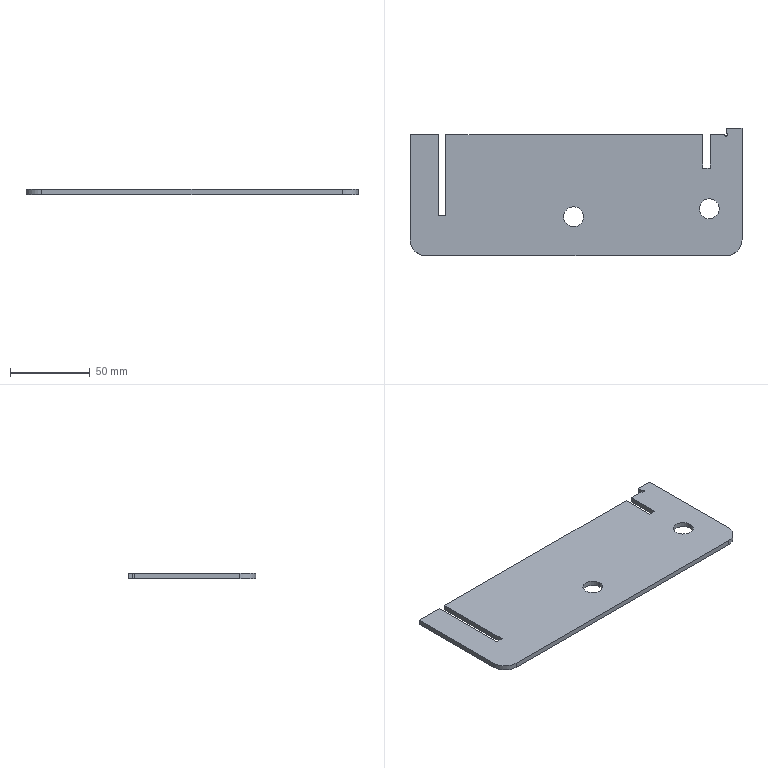Part | SolidWorks | features FlatPattern 1, SMBaseFlange 1, SheetMetal 1 | 1 solid | 23 faces | box 208 x 80 x 3.2 mm | volume 48747 mm3 | plane 16 | cylinder 7 | commonest cylinder face diameters 12.5 x4 20 x2 2 x1
STEP:
#1=CARTESIAN_POINT('',(88.351,-1041.506,3.2));
#2=VERTEX_POINT('',#1);
#3=CARTESIAN_POINT('',(100.851,-1041.506,3.2));
#4=VERTEX_POINT('',#3);
#5=CARTESIAN_POINT('',(94.601,-1041.506,3.2));
#6=DIRECTION('',(0.,0.,1.));
#7=DIRECTION('',(1.,0.,0.));
#8=AXIS2_PLACEMENT_3D('',#5,#6,#7);
#9=CIRCLE('',#8,6.25);
#10=EDGE_CURVE('',#2,#4,#9,.T.);
#11=ORIENTED_EDGE('',*,*,#10,.T.);
#12=CARTESIAN_POINT('',(100.851,-1041.506,0.));
#13=VERTEX_POINT('',#12);
#14=CARTESIAN_POINT('',(100.851,-1041.506,3.2));
#15=DIRECTION('',(0.,0.,-1.));
#16=VECTOR('',#15,1000.);
#17=LINE('',#14,#16);
#18=EDGE_CURVE('',#4,#13,#17,.T.);
#19=ORIENTED_EDGE('',*,*,#18,.T.);
#20=CARTESIAN_POINT('',(88.351,-1041.506,0.));
#21=VERTEX_POINT('',#20);
#22=CARTESIAN_POINT('',(94.601,-1041.506,0.));
#23=DIRECTION('',(0.,0.,1.));
#24=DIRECTION('',(1.,0.,0.));
#25=AXIS2_PLACEMENT_3D('',#22,#23,#24);
#26=CIRCLE('',#25,6.25);
#27=EDGE_CURVE('',#21,#13,#26,.T.);
#28=ORIENTED_EDGE('',*,*,#27,.F.);
#29=CARTESIAN_POINT('',(88.351,-1041.506,3.2));
#30=DIRECTION('',(0.,0.,-1.));
#31=VECTOR('',#30,1000.);
#32=LINE('',#29,#31);
#33=EDGE_CURVE('',#2,#21,#32,.T.);
#34=ORIENTED_EDGE('',*,*,#33,.F.);
#35=EDGE_LOOP('',(#11,#19,#28,#34));
#36=FACE_OUTER_BOUND('',#35,.T.);
#37=CARTESIAN_POINT('',(94.601,-1041.506,3.2));
#38=DIRECTION('',(0.,0.,-1.));
#39=DIRECTION('',(-1.,0.,0.));
#40=AXIS2_PLACEMENT_3D('',#37,#38,#39);
#41=CYLINDRICAL_SURFACE('',#40,6.25);
#42=ADVANCED_FACE('',(#36),#41,.F.);
#43=CARTESIAN_POINT('',(3.351,-1046.506,3.2));
#44=VERTEX_POINT('',#43);
#45=CARTESIAN_POINT('',(15.851,-1046.506,3.2));
#46=VERTEX_POINT('',#45);
#47=CARTESIAN_POINT('',(9.601,-1046.506,3.2));
#48=DIRECTION('',(0.,0.,1.));
#49=DIRECTION('',(1.,0.,0.));
#50=AXIS2_PLACEMENT_3D('',#47,#48,#49);
#51=CIRCLE('',#50,6.25);
#52=EDGE_CURVE('',#44,#46,#51,.T.);
#53=ORIENTED_EDGE('',*,*,#52,.T.);
#54=CARTESIAN_POINT('',(15.851,-1046.506,0.));
#55=VERTEX_POINT('',#54);
#56=CARTESIAN_POINT('',(15.851,-1046.506,3.2));
#57=DIRECTION('',(0.,0.,-1.));
#58=VECTOR('',#57,1000.);
#59=LINE('',#56,#58);
#60=EDGE_CURVE('',#46,#55,#59,.T.);
#61=ORIENTED_EDGE('',*,*,#60,.T.);
#62=CARTESIAN_POINT('',(3.351,-1046.506,0.));
#63=VERTEX_POINT('',#62);
#64=CARTESIAN_POINT('',(9.601,-1046.506,0.));
#65=DIRECTION('',(0.,0.,1.));
#66=DIRECTION('',(1.,0.,0.));
#67=AXIS2_PLACEMENT_3D('',#64,#65,#66);
#68=CIRCLE('',#67,6.25);
#69=EDGE_CURVE('',#63,#55,#68,.T.);
#70=ORIENTED_EDGE('',*,*,#69,.F.);
#71=CARTESIAN_POINT('',(3.351,-1046.506,3.2));
#72=DIRECTION('',(0.,0.,-1.));
#73=VECTOR('',#72,1000.);
#74=LINE('',#71,#73);
#75=EDGE_CURVE('',#44,#63,#74,.T.);
#76=ORIENTED_EDGE('',*,*,#75,.F.);
#77=EDGE_LOOP('',(#53,#61,#70,#76));
#78=FACE_OUTER_BOUND('',#77,.T.);
#79=CARTESIAN_POINT('',(9.601,-1046.506,3.2));
#80=DIRECTION('',(0.,0.,-1.));
#81=DIRECTION('',(-1.,0.,0.));
#82=AXIS2_PLACEMENT_3D('',#79,#80,#81);
#83=CYLINDRICAL_SURFACE('',#82,6.25);
#84=ADVANCED_FACE('',(#78),#83,.F.);
#85=ORIENTED_EDGE('',*,*,#52,.F.);
#86=CARTESIAN_POINT('',(9.601,-1046.506,3.2));
#87=DIRECTION('',(0.,0.,1.));
#88=DIRECTION('',(1.,0.,0.));
#89=AXIS2_PLACEMENT_3D('',#86,#87,#88);
#90=CIRCLE('',#89,6.25);
#91=EDGE_CURVE('',#46,#44,#90,.T.);
#92=ORIENTED_EDGE('',*,*,#91,.F.);
#93=EDGE_LOOP('',(#85,#92));
#94=FACE_BOUND('',#93,.T.);
#95=CARTESIAN_POINT('',(115.101,-991.006,3.2));
#96=VERTEX_POINT('',#95);
#97=CARTESIAN_POINT('',(105.101,-991.006,3.2));
#98=VERTEX_POINT('',#97);
#99=CARTESIAN_POINT('',(115.101,-991.006,3.2));
#100=DIRECTION('',(-1.,0.,0.));
#101=VECTOR('',#100,1000.);
#102=LINE('',#99,#101);
#103=EDGE_CURVE('',#96,#98,#102,.T.);
#104=ORIENTED_EDGE('',*,*,#103,.T.);
#105=CARTESIAN_POINT('',(105.101,-994.006,3.2));
#106=VERTEX_POINT('',#105);
#107=CARTESIAN_POINT('',(105.101,-991.006,3.2));
#108=DIRECTION('',(0.,-1.,0.));
#109=VECTOR('',#108,1000.);
#110=LINE('',#107,#109);
#111=EDGE_CURVE('',#98,#106,#110,.T.);
#112=ORIENTED_EDGE('',*,*,#111,.T.);
#113=CARTESIAN_POINT('',(104.101,-995.006,3.2));
#114=VERTEX_POINT('',#113);
#115=CARTESIAN_POINT('',(105.101,-995.006,3.2));
#116=DIRECTION('',(0.,0.,-1.));
#117=DIRECTION('',(1.,0.,0.));
#118=AXIS2_PLACEMENT_3D('',#115,#116,#117);
#119=CIRCLE('',#118,1.);
#120=EDGE_CURVE('',#106,#114,#119,.T.);
#121=ORIENTED_EDGE('',*,*,#120,.T.);
#122=CARTESIAN_POINT('',(95.101,-995.006,3.2));
#123=VERTEX_POINT('',#122);
#124=CARTESIAN_POINT('',(104.101,-995.006,3.2));
#125=DIRECTION('',(-1.,0.,0.));
#126=VECTOR('',#125,1000.);
#127=LINE('',#124,#126);
#128=EDGE_CURVE('',#114,#123,#127,.T.);
#129=ORIENTED_EDGE('',*,*,#128,.T.);
#130=CARTESIAN_POINT('',(95.101,-1016.006,3.2));
#131=VERTEX_POINT('',#130);
#132=CARTESIAN_POINT('',(95.101,-995.006,3.2));
#133=DIRECTION('',(0.,-1.,0.));
#134=VECTOR('',#133,1000.);
#135=LINE('',#132,#134);
#136=EDGE_CURVE('',#123,#131,#135,.T.);
#137=ORIENTED_EDGE('',*,*,#136,.T.);
#138=CARTESIAN_POINT('',(90.601,-1016.006,3.2));
#139=VERTEX_POINT('',#138);
#140=CARTESIAN_POINT('',(95.101,-1016.006,3.2));
#141=DIRECTION('',(-1.,0.,0.));
#142=VECTOR('',#141,1000.);
#143=LINE('',#140,#142);
#144=EDGE_CURVE('',#131,#139,#143,.T.);
#145=ORIENTED_EDGE('',*,*,#144,.T.);
#146=CARTESIAN_POINT('',(90.601,-995.006,3.2));
#147=VERTEX_POINT('',#146);
#148=CARTESIAN_POINT('',(90.601,-1016.006,3.2));
#149=DIRECTION('',(0.,1.,0.));
#150=VECTOR('',#149,1000.);
#151=LINE('',#148,#150);
#152=EDGE_CURVE('',#139,#147,#151,.T.);
#153=ORIENTED_EDGE('',*,*,#152,.T.);
#154=CARTESIAN_POINT('',(-70.399,-995.006,3.2));
#155=VERTEX_POINT('',#154);
#156=CARTESIAN_POINT('',(90.601,-995.006,3.2));
#157=DIRECTION('',(-1.,0.,0.));
#158=VECTOR('',#157,1000.);
#159=LINE('',#156,#158);
#160=EDGE_CURVE('',#147,#155,#159,.T.);
#161=ORIENTED_EDGE('',*,*,#160,.T.);
#162=CARTESIAN_POINT('',(-70.399,-1046.006,3.2));
#163=VERTEX_POINT('',#162);
#164=CARTESIAN_POINT('',(-70.399,-995.006,3.2));
#165=DIRECTION('',(0.,-1.,0.));
#166=VECTOR('',#165,1000.);
#167=LINE('',#164,#166);
#168=EDGE_CURVE('',#155,#163,#167,.T.);
#169=ORIENTED_EDGE('',*,*,#168,.T.);
#170=CARTESIAN_POINT('',(-74.899,-1046.006,3.2));
#171=VERTEX_POINT('',#170);
#172=CARTESIAN_POINT('',(-70.399,-1046.006,3.2));
#173=DIRECTION('',(-1.,0.,0.));
#174=VECTOR('',#173,1000.);
#175=LINE('',#172,#174);
#176=EDGE_CURVE('',#163,#171,#175,.T.);
#177=ORIENTED_EDGE('',*,*,#176,.T.);
#178=CARTESIAN_POINT('',(-74.899,-995.006,3.2));
#179=VERTEX_POINT('',#178);
#180=CARTESIAN_POINT('',(-74.899,-995.006,3.2));
#181=DIRECTION('',(0.,1.,0.));
#182=VECTOR('',#181,1000.);
#183=LINE('',#180,#182);
#184=EDGE_CURVE('',#171,#179,#183,.T.);
#185=ORIENTED_EDGE('',*,*,#184,.T.);
#186=CARTESIAN_POINT('',(-92.899,-995.006,3.2));
#187=VERTEX_POINT('',#186);
#188=CARTESIAN_POINT('',(-74.899,-995.006,3.2));
#189=DIRECTION('',(-1.,0.,0.));
#190=VECTOR('',#189,1000.);
#191=LINE('',#188,#190);
#192=EDGE_CURVE('',#179,#187,#191,.T.);
#193=ORIENTED_EDGE('',*,*,#192,.T.);
#194=CARTESIAN_POINT('',(-92.899,-1061.006,3.2));
#195=VERTEX_POINT('',#194);
#196=CARTESIAN_POINT('',(-92.899,-995.006,3.2));
#197=DIRECTION('',(0.,-1.,0.));
#198=VECTOR('',#197,1000.);
#199=LINE('',#196,#198);
#200=EDGE_CURVE('',#187,#195,#199,.T.);
#201=ORIENTED_EDGE('',*,*,#200,.T.);
#202=CARTESIAN_POINT('',(-82.899,-1071.006,3.2));
#203=VERTEX_POINT('',#202);
#204=CARTESIAN_POINT('',(-82.899,-1061.006,3.2));
#205=DIRECTION('',(0.,0.,1.));
#206=DIRECTION('',(1.,0.,0.));
#207=AXIS2_PLACEMENT_3D('',#204,#205,#206);
#208=CIRCLE('',#207,10.);
#209=EDGE_CURVE('',#195,#203,#208,.T.);
#210=ORIENTED_EDGE('',*,*,#209,.T.);
#211=CARTESIAN_POINT('',(105.101,-1071.006,3.2));
#212=VERTEX_POINT('',#211);
#213=CARTESIAN_POINT('',(-82.899,-1071.006,3.2));
#214=DIRECTION('',(1.,0.,0.));
#215=VECTOR('',#214,1000.);
#216=LINE('',#213,#215);
#217=EDGE_CURVE('',#203,#212,#216,.T.);
#218=ORIENTED_EDGE('',*,*,#217,.T.);
#219=CARTESIAN_POINT('',(115.101,-1061.006,3.2));
#220=VERTEX_POINT('',#219);
#221=CARTESIAN_POINT('',(105.101,-1061.006,3.2));
#222=DIRECTION('',(0.,0.,1.));
#223=DIRECTION('',(1.,0.,0.));
#224=AXIS2_PLACEMENT_3D('',#221,#222,#223);
#225=CIRCLE('',#224,10.);
#226=EDGE_CURVE('',#212,#220,#225,.T.);
#227=ORIENTED_EDGE('',*,*,#226,.T.);
#228=CARTESIAN_POINT('',(115.101,-1061.006,3.2));
#229=DIRECTION('',(0.,1.,0.));
#230=VECTOR('',#229,1000.);
#231=LINE('',#228,#230);
#232=EDGE_CURVE('',#220,#96,#231,.T.);
#233=ORIENTED_EDGE('',*,*,#232,.T.);
#234=EDGE_LOOP('',(#104,#112,#121,#129,#137,#145,#153,#161,#169,#177,#185,#193,#201,#210,#218,#227,#233));
#235=FACE_OUTER_BOUND('',#234,.T.);
#236=ORIENTED_EDGE('',*,*,#10,.F.);
#237=CARTESIAN_POINT('',(94.601,-1041.506,3.2));
#238=DIRECTION('',(0.,0.,1.));
#239=DIRECTION('',(1.,0.,0.));
#240=AXIS2_PLACEMENT_3D('',#237,#238,#239);
#241=CIRCLE('',#240,6.25);
#242=EDGE_CURVE('',#4,#2,#241,.T.);
#243=ORIENTED_EDGE('',*,*,#242,.F.);
#244=EDGE_LOOP('',(#236,#243));
#245=FACE_BOUND('',#244,.T.);
#246=CARTESIAN_POINT('',(105.101,-995.006,3.2));
#247=DIRECTION('',(0.,0.,1.));
#248=DIRECTION('',(1.,0.,0.));
#249=AXIS2_PLACEMENT_3D('',#246,#247,#248);
#250=PLANE('',#249);
#251=ADVANCED_FACE('',(#94,#235,#245),#250,.T.);
#252=CARTESIAN_POINT('',(115.101,-991.006,0.));
#253=VERTEX_POINT('',#252);
#254=CARTESIAN_POINT('',(105.101,-991.006,0.));
#255=VERTEX_POINT('',#254);
#256=CARTESIAN_POINT('',(115.101,-991.006,0.));
#257=DIRECTION('',(-1.,0.,0.));
#258=VECTOR('',#257,1000.);
#259=LINE('',#256,#258);
#260=EDGE_CURVE('',#253,#255,#259,.T.);
#261=ORIENTED_EDGE('',*,*,#260,.F.);
#262=CARTESIAN_POINT('',(115.101,-1061.006,0.));
#263=VERTEX_POINT('',#262);
#264=CARTESIAN_POINT('',(115.101,-1061.006,0.));
#265=DIRECTION('',(0.,1.,0.));
#266=VECTOR('',#265,1000.);
#267=LINE('',#264,#266);
#268=EDGE_CURVE('',#263,#253,#267,.T.);
#269=ORIENTED_EDGE('',*,*,#268,.F.);
#270=CARTESIAN_POINT('',(105.101,-1071.006,0.));
#271=VERTEX_POINT('',#270);
#272=CARTESIAN_POINT('',(105.101,-1061.006,0.));
#273=DIRECTION('',(0.,0.,1.));
#274=DIRECTION('',(1.,0.,0.));
#275=AXIS2_PLACEMENT_3D('',#272,#273,#274);
#276=CIRCLE('',#275,10.);
#277=EDGE_CURVE('',#271,#263,#276,.T.);
#278=ORIENTED_EDGE('',*,*,#277,.F.);
#279=CARTESIAN_POINT('',(-82.899,-1071.006,0.));
#280=VERTEX_POINT('',#279);
#281=CARTESIAN_POINT('',(-82.899,-1071.006,0.));
#282=DIRECTION('',(1.,0.,0.));
#283=VECTOR('',#282,1000.);
#284=LINE('',#281,#283);
#285=EDGE_CURVE('',#280,#271,#284,.T.);
#286=ORIENTED_EDGE('',*,*,#285,.F.);
#287=CARTESIAN_POINT('',(-92.899,-1061.006,0.));
#288=VERTEX_POINT('',#287);
#289=CARTESIAN_POINT('',(-82.899,-1061.006,0.));
#290=DIRECTION('',(0.,0.,1.));
#291=DIRECTION('',(1.,0.,0.));
#292=AXIS2_PLACEMENT_3D('',#289,#290,#291);
#293=CIRCLE('',#292,10.);
#294=EDGE_CURVE('',#288,#280,#293,.T.);
#295=ORIENTED_EDGE('',*,*,#294,.F.);
#296=CARTESIAN_POINT('',(-92.899,-995.006,0.));
#297=VERTEX_POINT('',#296);
#298=CARTESIAN_POINT('',(-92.899,-995.006,0.));
#299=DIRECTION('',(0.,-1.,0.));
#300=VECTOR('',#299,1000.);
#301=LINE('',#298,#300);
#302=EDGE_CURVE('',#297,#288,#301,.T.);
#303=ORIENTED_EDGE('',*,*,#302,.F.);
#304=CARTESIAN_POINT('',(-74.899,-995.006,0.));
#305=VERTEX_POINT('',#304);
#306=CARTESIAN_POINT('',(-74.899,-995.006,0.));
#307=DIRECTION('',(-1.,0.,0.));
#308=VECTOR('',#307,1000.);
#309=LINE('',#306,#308);
#310=EDGE_CURVE('',#305,#297,#309,.T.);
#311=ORIENTED_EDGE('',*,*,#310,.F.);
#312=CARTESIAN_POINT('',(-74.899,-1046.006,0.));
#313=VERTEX_POINT('',#312);
#314=CARTESIAN_POINT('',(-74.899,-995.006,0.));
#315=DIRECTION('',(0.,1.,0.));
#316=VECTOR('',#315,1000.);
#317=LINE('',#314,#316);
#318=EDGE_CURVE('',#313,#305,#317,.T.);
#319=ORIENTED_EDGE('',*,*,#318,.F.);
#320=CARTESIAN_POINT('',(-70.399,-1046.006,0.));
#321=VERTEX_POINT('',#320);
#322=CARTESIAN_POINT('',(-70.399,-1046.006,0.));
#323=DIRECTION('',(-1.,0.,0.));
#324=VECTOR('',#323,1000.);
#325=LINE('',#322,#324);
#326=EDGE_CURVE('',#321,#313,#325,.T.);
#327=ORIENTED_EDGE('',*,*,#326,.F.);
#328=CARTESIAN_POINT('',(-70.399,-995.006,0.));
#329=VERTEX_POINT('',#328);
#330=CARTESIAN_POINT('',(-70.399,-995.006,0.));
#331=DIRECTION('',(0.,-1.,0.));
#332=VECTOR('',#331,1000.);
#333=LINE('',#330,#332);
#334=EDGE_CURVE('',#329,#321,#333,.T.);
#335=ORIENTED_EDGE('',*,*,#334,.F.);
#336=CARTESIAN_POINT('',(90.601,-995.006,0.));
#337=VERTEX_POINT('',#336);
#338=CARTESIAN_POINT('',(90.601,-995.006,0.));
#339=DIRECTION('',(-1.,0.,0.));
#340=VECTOR('',#339,1000.);
#341=LINE('',#338,#340);
#342=EDGE_CURVE('',#337,#329,#341,.T.);
#343=ORIENTED_EDGE('',*,*,#342,.F.);
#344=CARTESIAN_POINT('',(90.601,-1016.006,0.));
#345=VERTEX_POINT('',#344);
#346=CARTESIAN_POINT('',(90.601,-1016.006,0.));
#347=DIRECTION('',(0.,1.,0.));
#348=VECTOR('',#347,1000.);
#349=LINE('',#346,#348);
#350=EDGE_CURVE('',#345,#337,#349,.T.);
#351=ORIENTED_EDGE('',*,*,#350,.F.);
#352=CARTESIAN_POINT('',(95.101,-1016.006,0.));
#353=VERTEX_POINT('',#352);
#354=CARTESIAN_POINT('',(95.101,-1016.006,0.));
#355=DIRECTION('',(-1.,0.,0.));
#356=VECTOR('',#355,1000.);
#357=LINE('',#354,#356);
#358=EDGE_CURVE('',#353,#345,#357,.T.);
#359=ORIENTED_EDGE('',*,*,#358,.F.);
#360=CARTESIAN_POINT('',(95.101,-995.006,0.));
#361=VERTEX_POINT('',#360);
#362=CARTESIAN_POINT('',(95.101,-995.006,0.));
#363=DIRECTION('',(0.,-1.,0.));
#364=VECTOR('',#363,1000.);
#365=LINE('',#362,#364);
#366=EDGE_CURVE('',#361,#353,#365,.T.);
#367=ORIENTED_EDGE('',*,*,#366,.F.);
#368=CARTESIAN_POINT('',(104.101,-995.006,0.));
#369=VERTEX_POINT('',#368);
#370=CARTESIAN_POINT('',(104.101,-995.006,0.));
#371=DIRECTION('',(-1.,0.,0.));
#372=VECTOR('',#371,1000.);
#373=LINE('',#370,#372);
#374=EDGE_CURVE('',#369,#361,#373,.T.);
#375=ORIENTED_EDGE('',*,*,#374,.F.);
#376=CARTESIAN_POINT('',(105.101,-994.006,0.));
#377=VERTEX_POINT('',#376);
#378=CARTESIAN_POINT('',(105.101,-995.006,0.));
#379=DIRECTION('',(0.,0.,-1.));
#380=DIRECTION('',(1.,0.,0.));
#381=AXIS2_PLACEMENT_3D('',#378,#379,#380);
#382=CIRCLE('',#381,1.);
#383=EDGE_CURVE('',#377,#369,#382,.T.);
#384=ORIENTED_EDGE('',*,*,#383,.F.);
#385=CARTESIAN_POINT('',(105.101,-991.006,0.));
#386=DIRECTION('',(0.,-1.,0.));
#387=VECTOR('',#386,1000.);
#388=LINE('',#385,#387);
#389=EDGE_CURVE('',#255,#377,#388,.T.);
#390=ORIENTED_EDGE('',*,*,#389,.F.);
#391=EDGE_LOOP('',(#261,#269,#278,#286,#295,#303,#311,#319,#327,#335,#343,#351,#359,#367,#375,#384,#390));
#392=FACE_OUTER_BOUND('',#391,.T.);
#393=ORIENTED_EDGE('',*,*,#69,.T.);
#394=CARTESIAN_POINT('',(9.601,-1046.506,0.));
#395=DIRECTION('',(0.,0.,1.));
#396=DIRECTION('',(1.,0.,0.));
#397=AXIS2_PLACEMENT_3D('',#394,#395,#396);
#398=CIRCLE('',#397,6.25);
#399=EDGE_CURVE('',#55,#63,#398,.T.);
#400=ORIENTED_EDGE('',*,*,#399,.T.);
#401=EDGE_LOOP('',(#393,#400));
#402=FACE_BOUND('',#401,.T.);
#403=ORIENTED_EDGE('',*,*,#27,.T.);
#404=CARTESIAN_POINT('',(94.601,-1041.506,0.));
#405=DIRECTION('',(0.,0.,1.));
#406=DIRECTION('',(1.,0.,0.));
#407=AXIS2_PLACEMENT_3D('',#404,#405,#406);
#408=CIRCLE('',#407,6.25);
#409=EDGE_CURVE('',#13,#21,#408,.T.);
#410=ORIENTED_EDGE('',*,*,#409,.T.);
#411=EDGE_LOOP('',(#403,#410));
#412=FACE_BOUND('',#411,.T.);
#413=CARTESIAN_POINT('',(105.101,-995.006,0.));
#414=DIRECTION('',(0.,0.,1.));
#415=DIRECTION('',(1.,0.,0.));
#416=AXIS2_PLACEMENT_3D('',#413,#414,#415);
#417=PLANE('',#416);
#418=ADVANCED_FACE('',(#392,#402,#412),#417,.F.);
#419=ORIENTED_EDGE('',*,*,#260,.T.);
#420=CARTESIAN_POINT('',(105.101,-991.006,3.2));
#421=DIRECTION('',(0.,0.,-1.));
#422=VECTOR('',#421,1000.);
#423=LINE('',#420,#422);
#424=EDGE_CURVE('',#98,#255,#423,.T.);
#425=ORIENTED_EDGE('',*,*,#424,.F.);
#426=ORIENTED_EDGE('',*,*,#103,.F.);
#427=CARTESIAN_POINT('',(115.101,-991.006,3.2));
#428=DIRECTION('',(0.,0.,-1.));
#429=VECTOR('',#428,1000.);
#430=LINE('',#427,#429);
#431=EDGE_CURVE('',#96,#253,#430,.T.);
#432=ORIENTED_EDGE('',*,*,#431,.T.);
#433=EDGE_LOOP('',(#419,#425,#426,#432));
#434=FACE_OUTER_BOUND('',#433,.T.);
#435=CARTESIAN_POINT('',(115.101,-991.006,3.2));
#436=DIRECTION('',(0.,-1.,0.));
#437=DIRECTION('',(0.,0.,-1.));
#438=AXIS2_PLACEMENT_3D('',#435,#436,#437);
#439=PLANE('',#438);
#440=ADVANCED_FACE('',(#434),#439,.F.);
#441=ORIENTED_EDGE('',*,*,#389,.T.);
#442=CARTESIAN_POINT('',(105.101,-994.006,3.2));
#443=DIRECTION('',(0.,0.,-1.));
#444=VECTOR('',#443,1000.);
#445=LINE('',#442,#444);
#446=EDGE_CURVE('',#106,#377,#445,.T.);
#447=ORIENTED_EDGE('',*,*,#446,.F.);
#448=ORIENTED_EDGE('',*,*,#111,.F.);
#449=ORIENTED_EDGE('',*,*,#424,.T.);
#450=EDGE_LOOP('',(#441,#447,#448,#449));
#451=FACE_OUTER_BOUND('',#450,.T.);
#452=CARTESIAN_POINT('',(105.101,-991.006,3.2));
#453=DIRECTION('',(1.,0.,0.));
#454=DIRECTION('',(0.,0.,-1.));
#455=AXIS2_PLACEMENT_3D('',#452,#453,#454);
#456=PLANE('',#455);
#457=ADVANCED_FACE('',(#451),#456,.F.);
#458=ORIENTED_EDGE('',*,*,#383,.T.);
#459=CARTESIAN_POINT('',(104.101,-995.006,3.2));
#460=DIRECTION('',(0.,0.,-1.));
#461=VECTOR('',#460,1000.);
#462=LINE('',#459,#461);
#463=EDGE_CURVE('',#114,#369,#462,.T.);
#464=ORIENTED_EDGE('',*,*,#463,.F.);
#465=ORIENTED_EDGE('',*,*,#120,.F.);
#466=ORIENTED_EDGE('',*,*,#446,.T.);
#467=EDGE_LOOP('',(#458,#464,#465,#466));
#468=FACE_OUTER_BOUND('',#467,.T.);
#469=CARTESIAN_POINT('',(105.101,-995.006,3.2));
#470=DIRECTION('',(0.,0.,-1.));
#471=DIRECTION('',(-1.,0.,0.));
#472=AXIS2_PLACEMENT_3D('',#469,#470,#471);
#473=CYLINDRICAL_SURFACE('',#472,1.);
#474=ADVANCED_FACE('',(#468),#473,.F.);
#475=ORIENTED_EDGE('',*,*,#374,.T.);
#476=CARTESIAN_POINT('',(95.101,-995.006,3.2));
#477=DIRECTION('',(0.,0.,-1.));
#478=VECTOR('',#477,1000.);
#479=LINE('',#476,#478);
#480=EDGE_CURVE('',#123,#361,#479,.T.);
#481=ORIENTED_EDGE('',*,*,#480,.F.);
#482=ORIENTED_EDGE('',*,*,#128,.F.);
#483=ORIENTED_EDGE('',*,*,#463,.T.);
#484=EDGE_LOOP('',(#475,#481,#482,#483));
#485=FACE_OUTER_BOUND('',#484,.T.);
#486=CARTESIAN_POINT('',(104.101,-995.006,3.2));
#487=DIRECTION('',(0.,-1.,0.));
#488=DIRECTION('',(1.,0.,0.));
#489=AXIS2_PLACEMENT_3D('',#486,#487,#488);
#490=PLANE('',#489);
#491=ADVANCED_FACE('',(#485),#490,.F.);
#492=ORIENTED_EDGE('',*,*,#366,.T.);
#493=CARTESIAN_POINT('',(95.101,-1016.006,3.2));
#494=DIRECTION('',(0.,0.,-1.));
#495=VECTOR('',#494,1000.);
#496=LINE('',#493,#495);
#497=EDGE_CURVE('',#131,#353,#496,.T.);
#498=ORIENTED_EDGE('',*,*,#497,.F.);
#499=ORIENTED_EDGE('',*,*,#136,.F.);
#500=ORIENTED_EDGE('',*,*,#480,.T.);
#501=EDGE_LOOP('',(#492,#498,#499,#500));
#502=FACE_OUTER_BOUND('',#501,.T.);
#503=CARTESIAN_POINT('',(95.101,-995.006,3.2));
#504=DIRECTION('',(1.,0.,0.));
#505=DIRECTION('',(0.,1.,0.));
#506=AXIS2_PLACEMENT_3D('',#503,#504,#505);
#507=PLANE('',#506);
#508=ADVANCED_FACE('',(#502),#507,.F.);
#509=ORIENTED_EDGE('',*,*,#358,.T.);
#510=CARTESIAN_POINT('',(90.601,-1016.006,3.2));
#511=DIRECTION('',(0.,0.,-1.));
#512=VECTOR('',#511,1000.);
#513=LINE('',#510,#512);
#514=EDGE_CURVE('',#139,#345,#513,.T.);
#515=ORIENTED_EDGE('',*,*,#514,.F.);
#516=ORIENTED_EDGE('',*,*,#144,.F.);
#517=ORIENTED_EDGE('',*,*,#497,.T.);
#518=EDGE_LOOP('',(#509,#515,#516,#517));
#519=FACE_OUTER_BOUND('',#518,.T.);
#520=CARTESIAN_POINT('',(95.101,-1016.006,3.2));
#521=DIRECTION('',(0.,-1.,0.));
#522=DIRECTION('',(0.,0.,-1.));
#523=AXIS2_PLACEMENT_3D('',#520,#521,#522);
#524=PLANE('',#523);
#525=ADVANCED_FACE('',(#519),#524,.F.);
#526=ORIENTED_EDGE('',*,*,#350,.T.);
#527=CARTESIAN_POINT('',(90.601,-995.006,3.2));
#528=DIRECTION('',(0.,0.,-1.));
#529=VECTOR('',#528,1000.);
#530=LINE('',#527,#529);
#531=EDGE_CURVE('',#147,#337,#530,.T.);
#532=ORIENTED_EDGE('',*,*,#531,.F.);
#533=ORIENTED_EDGE('',*,*,#152,.F.);
#534=ORIENTED_EDGE('',*,*,#514,.T.);
#535=EDGE_LOOP('',(#526,#532,#533,#534));
#536=FACE_OUTER_BOUND('',#535,.T.);
#537=CARTESIAN_POINT('',(90.601,-1016.006,3.2));
#538=DIRECTION('',(-1.,0.,0.));
#539=DIRECTION('',(0.,0.,1.));
#540=AXIS2_PLACEMENT_3D('',#537,#538,#539);
#541=PLANE('',#540);
#542=ADVANCED_FACE('',(#536),#541,.F.);
#543=ORIENTED_EDGE('',*,*,#342,.T.);
#544=CARTESIAN_POINT('',(-70.399,-995.006,3.2));
#545=DIRECTION('',(0.,0.,-1.));
#546=VECTOR('',#545,1000.);
#547=LINE('',#544,#546);
#548=EDGE_CURVE('',#155,#329,#547,.T.);
#549=ORIENTED_EDGE('',*,*,#548,.F.);
#550=ORIENTED_EDGE('',*,*,#160,.F.);
#551=ORIENTED_EDGE('',*,*,#531,.T.);
#552=EDGE_LOOP('',(#543,#549,#550,#551));
#553=FACE_OUTER_BOUND('',#552,.T.);
#554=CARTESIAN_POINT('',(90.601,-995.006,3.2));
#555=DIRECTION('',(0.,-1.,0.));
#556=DIRECTION('',(1.,0.,0.));
#557=AXIS2_PLACEMENT_3D('',#554,#555,#556);
#558=PLANE('',#557);
#559=ADVANCED_FACE('',(#553),#558,.F.);
#560=ORIENTED_EDGE('',*,*,#334,.T.);
#561=CARTESIAN_POINT('',(-70.399,-1046.006,3.2));
#562=DIRECTION('',(0.,0.,-1.));
#563=VECTOR('',#562,1000.);
#564=LINE('',#561,#563);
#565=EDGE_CURVE('',#163,#321,#564,.T.);
#566=ORIENTED_EDGE('',*,*,#565,.F.);
#567=ORIENTED_EDGE('',*,*,#168,.F.);
#568=ORIENTED_EDGE('',*,*,#548,.T.);
#569=EDGE_LOOP('',(#560,#566,#567,#568));
#570=FACE_OUTER_BOUND('',#569,.T.);
#571=CARTESIAN_POINT('',(-70.399,-995.006,3.2));
#572=DIRECTION('',(1.,0.,0.));
#573=DIRECTION('',(0.,0.,-1.));
#574=AXIS2_PLACEMENT_3D('',#571,#572,#573);
#575=PLANE('',#574);
#576=ADVANCED_FACE('',(#570),#575,.F.);
#577=ORIENTED_EDGE('',*,*,#326,.T.);
#578=CARTESIAN_POINT('',(-74.899,-1046.006,3.2));
#579=DIRECTION('',(0.,0.,-1.));
#580=VECTOR('',#579,1000.);
#581=LINE('',#578,#580);
#582=EDGE_CURVE('',#171,#313,#581,.T.);
#583=ORIENTED_EDGE('',*,*,#582,.F.);
#584=ORIENTED_EDGE('',*,*,#176,.F.);
#585=ORIENTED_EDGE('',*,*,#565,.T.);
#586=EDGE_LOOP('',(#577,#583,#584,#585));
#587=FACE_OUTER_BOUND('',#586,.T.);
#588=CARTESIAN_POINT('',(-70.399,-1046.006,3.2));
#589=DIRECTION('',(0.,-1.,0.));
#590=DIRECTION('',(0.,0.,-1.));
#591=AXIS2_PLACEMENT_3D('',#588,#589,#590);
#592=PLANE('',#591);
#593=ADVANCED_FACE('',(#587),#592,.F.);
#594=ORIENTED_EDGE('',*,*,#318,.T.);
#595=CARTESIAN_POINT('',(-74.899,-995.006,3.2));
#596=DIRECTION('',(0.,0.,-1.));
#597=VECTOR('',#596,1000.);
#598=LINE('',#595,#597);
#599=EDGE_CURVE('',#179,#305,#598,.T.);
#600=ORIENTED_EDGE('',*,*,#599,.F.);
#601=ORIENTED_EDGE('',*,*,#184,.F.);
#602=ORIENTED_EDGE('',*,*,#582,.T.);
#603=EDGE_LOOP('',(#594,#600,#601,#602));
#604=FACE_OUTER_BOUND('',#603,.T.);
#605=CARTESIAN_POINT('',(-74.899,-995.006,3.2));
#606=DIRECTION('',(-1.,0.,0.));
#607=DIRECTION('',(0.,0.,1.));
#608=AXIS2_PLACEMENT_3D('',#605,#606,#607);
#609=PLANE('',#608);
#610=ADVANCED_FACE('',(#604),#609,.F.);
#611=ORIENTED_EDGE('',*,*,#310,.T.);
#612=CARTESIAN_POINT('',(-92.899,-995.006,3.2));
#613=DIRECTION('',(0.,0.,-1.));
#614=VECTOR('',#613,1000.);
#615=LINE('',#612,#614);
#616=EDGE_CURVE('',#187,#297,#615,.T.);
#617=ORIENTED_EDGE('',*,*,#616,.F.);
#618=ORIENTED_EDGE('',*,*,#192,.F.);
#619=ORIENTED_EDGE('',*,*,#599,.T.);
#620=EDGE_LOOP('',(#611,#617,#618,#619));
#621=FACE_OUTER_BOUND('',#620,.T.);
#622=CARTESIAN_POINT('',(-74.899,-995.006,3.2));
#623=DIRECTION('',(0.,-1.,0.));
#624=DIRECTION('',(1.,0.,0.));
#625=AXIS2_PLACEMENT_3D('',#622,#623,#624);
#626=PLANE('',#625);
#627=ADVANCED_FACE('',(#621),#626,.F.);
#628=ORIENTED_EDGE('',*,*,#302,.T.);
#629=CARTESIAN_POINT('',(-92.899,-1061.006,3.2));
#630=DIRECTION('',(0.,0.,-1.));
#631=VECTOR('',#630,1000.);
#632=LINE('',#629,#631);
#633=EDGE_CURVE('',#195,#288,#632,.T.);
#634=ORIENTED_EDGE('',*,*,#633,.F.);
#635=ORIENTED_EDGE('',*,*,#200,.F.);
#636=ORIENTED_EDGE('',*,*,#616,.T.);
#637=EDGE_LOOP('',(#628,#634,#635,#636));
#638=FACE_OUTER_BOUND('',#637,.T.);
#639=CARTESIAN_POINT('',(-92.899,-995.006,3.2));
#640=DIRECTION('',(1.,0.,0.));
#641=DIRECTION('',(0.,0.,-1.));
#642=AXIS2_PLACEMENT_3D('',#639,#640,#641);
#643=PLANE('',#642);
#644=ADVANCED_FACE('',(#638),#643,.F.);
#645=ORIENTED_EDGE('',*,*,#294,.T.);
#646=CARTESIAN_POINT('',(-82.899,-1071.006,3.2));
#647=DIRECTION('',(0.,0.,-1.));
#648=VECTOR('',#647,1000.);
#649=LINE('',#646,#648);
#650=EDGE_CURVE('',#203,#280,#649,.T.);
#651=ORIENTED_EDGE('',*,*,#650,.F.);
#652=ORIENTED_EDGE('',*,*,#209,.F.);
#653=ORIENTED_EDGE('',*,*,#633,.T.);
#654=EDGE_LOOP('',(#645,#651,#652,#653));
#655=FACE_OUTER_BOUND('',#654,.T.);
#656=CARTESIAN_POINT('',(-82.899,-1061.006,3.2));
#657=DIRECTION('',(0.,0.,-1.));
#658=DIRECTION('',(-1.,0.,0.));
#659=AXIS2_PLACEMENT_3D('',#656,#657,#658);
#660=CYLINDRICAL_SURFACE('',#659,10.);
#661=ADVANCED_FACE('',(#655),#660,.T.);
#662=ORIENTED_EDGE('',*,*,#285,.T.);
#663=CARTESIAN_POINT('',(105.101,-1071.006,3.2));
#664=DIRECTION('',(0.,0.,-1.));
#665=VECTOR('',#664,1000.);
#666=LINE('',#663,#665);
#667=EDGE_CURVE('',#212,#271,#666,.T.);
#668=ORIENTED_EDGE('',*,*,#667,.F.);
#669=ORIENTED_EDGE('',*,*,#217,.F.);
#670=ORIENTED_EDGE('',*,*,#650,.T.);
#671=EDGE_LOOP('',(#662,#668,#669,#670));
#672=FACE_OUTER_BOUND('',#671,.T.);
#673=CARTESIAN_POINT('',(-82.899,-1071.006,3.2));
#674=DIRECTION('',(0.,1.,0.));
#675=DIRECTION('',(0.,0.,1.));
#676=AXIS2_PLACEMENT_3D('',#673,#674,#675);
#677=PLANE('',#676);
#678=ADVANCED_FACE('',(#672),#677,.F.);
#679=ORIENTED_EDGE('',*,*,#277,.T.);
#680=CARTESIAN_POINT('',(115.101,-1061.006,3.2));
#681=DIRECTION('',(0.,0.,-1.));
#682=VECTOR('',#681,1000.);
#683=LINE('',#680,#682);
#684=EDGE_CURVE('',#220,#263,#683,.T.);
#685=ORIENTED_EDGE('',*,*,#684,.F.);
#686=ORIENTED_EDGE('',*,*,#226,.F.);
#687=ORIENTED_EDGE('',*,*,#667,.T.);
#688=EDGE_LOOP('',(#679,#685,#686,#687));
#689=FACE_OUTER_BOUND('',#688,.T.);
#690=CARTESIAN_POINT('',(105.101,-1061.006,3.2));
#691=DIRECTION('',(0.,0.,-1.));
#692=DIRECTION('',(-1.,0.,0.));
#693=AXIS2_PLACEMENT_3D('',#690,#691,#692);
#694=CYLINDRICAL_SURFACE('',#693,10.);
#695=ADVANCED_FACE('',(#689),#694,.T.);
#696=ORIENTED_EDGE('',*,*,#268,.T.);
#697=ORIENTED_EDGE('',*,*,#431,.F.);
#698=ORIENTED_EDGE('',*,*,#232,.F.);
#699=ORIENTED_EDGE('',*,*,#684,.T.);
#700=EDGE_LOOP('',(#696,#697,#698,#699));
#701=FACE_OUTER_BOUND('',#700,.T.);
#702=CARTESIAN_POINT('',(115.101,-1061.006,3.2));
#703=DIRECTION('',(-1.,0.,0.));
#704=DIRECTION('',(0.,0.,1.));
#705=AXIS2_PLACEMENT_3D('',#702,#703,#704);
#706=PLANE('',#705);
#707=ADVANCED_FACE('',(#701),#706,.F.);
#708=ORIENTED_EDGE('',*,*,#60,.F.);
#709=ORIENTED_EDGE('',*,*,#91,.T.);
#710=ORIENTED_EDGE('',*,*,#75,.T.);
#711=ORIENTED_EDGE('',*,*,#399,.F.);
#712=EDGE_LOOP('',(#708,#709,#710,#711));
#713=FACE_OUTER_BOUND('',#712,.T.);
#714=CARTESIAN_POINT('',(9.601,-1046.506,3.2));
#715=DIRECTION('',(0.,0.,-1.));
#716=DIRECTION('',(-1.,0.,0.));
#717=AXIS2_PLACEMENT_3D('',#714,#715,#716);
#718=CYLINDRICAL_SURFACE('',#717,6.25);
#719=ADVANCED_FACE('',(#713),#718,.F.);
#720=ORIENTED_EDGE('',*,*,#18,.F.);
#721=ORIENTED_EDGE('',*,*,#242,.T.);
#722=ORIENTED_EDGE('',*,*,#33,.T.);
#723=ORIENTED_EDGE('',*,*,#409,.F.);
#724=EDGE_LOOP('',(#720,#721,#722,#723));
#725=FACE_OUTER_BOUND('',#724,.T.);
#726=CARTESIAN_POINT('',(94.601,-1041.506,3.2));
#727=DIRECTION('',(0.,0.,-1.));
#728=DIRECTION('',(-1.,0.,0.));
#729=AXIS2_PLACEMENT_3D('',#726,#727,#728);
#730=CYLINDRICAL_SURFACE('',#729,6.25);
#731=ADVANCED_FACE('',(#725),#730,.F.);
#732=CLOSED_SHELL('',(#42,#84,#251,#418,#440,#457,#474,#491,#508,#525,#542,#559,#576,#593,#610,#627,#644,#661,#678,#695,#707,#719,#731));
#733=MANIFOLD_SOLID_BREP('',#732);
#734=CARTESIAN_POINT('',(0.,0.,0.));
#735=DIRECTION('',(0.,0.,1.));
#736=DIRECTION('',(1.,0.,0.));
#737=AXIS2_PLACEMENT_3D('',#734,#735,#736);
#738=(LENGTH_UNIT()NAMED_UNIT(*)SI_UNIT(.MILLI.,.METRE.));
#739=UNCERTAINTY_MEASURE_WITH_UNIT(LENGTH_MEASURE(0.00001),#738,'','');
#740=(NAMED_UNIT(*)PLANE_ANGLE_UNIT()SI_UNIT($,.RADIAN.));
#741=(NAMED_UNIT(*)SI_UNIT($,.STERADIAN.)SOLID_ANGLE_UNIT());
#742=(GEOMETRIC_REPRESENTATION_CONTEXT(3)GLOBAL_UNCERTAINTY_ASSIGNED_CONTEXT((#739))GLOBAL_UNIT_ASSIGNED_CONTEXT((#738,#740,#741))REPRESENTATION_CONTEXT('',''));
#743=ADVANCED_BREP_SHAPE_REPRESENTATION('',(#733,#737),#742);